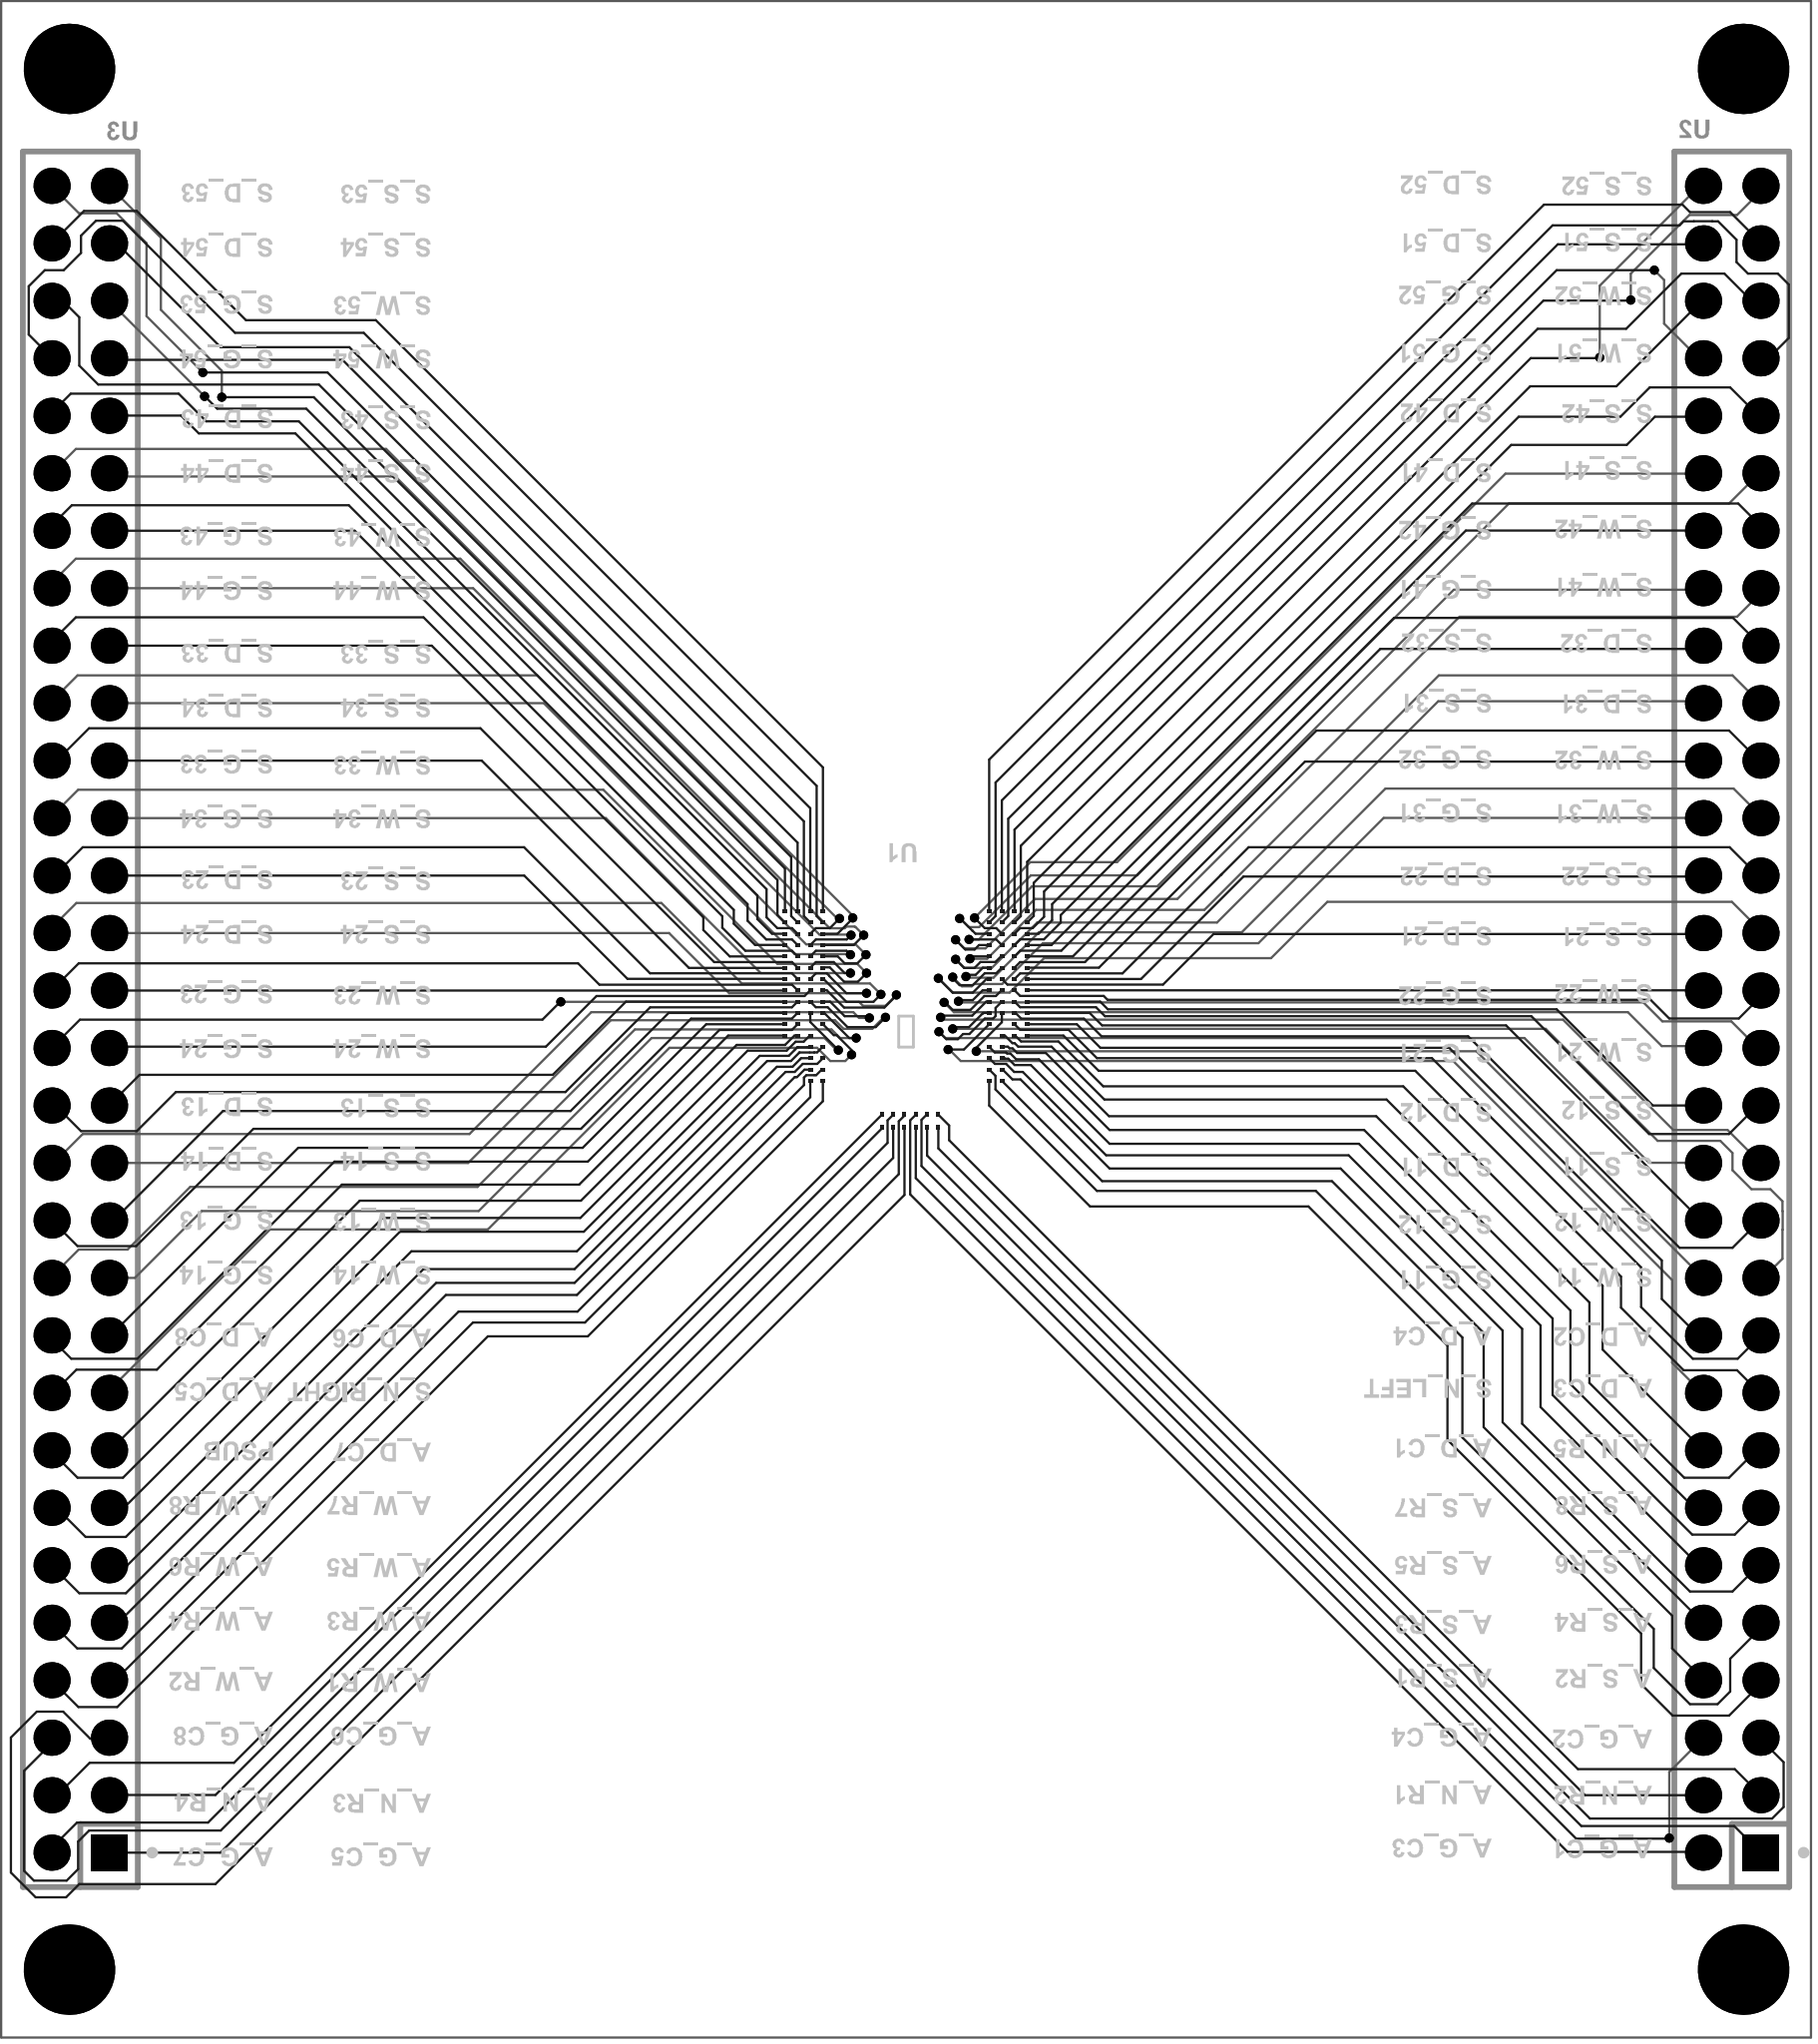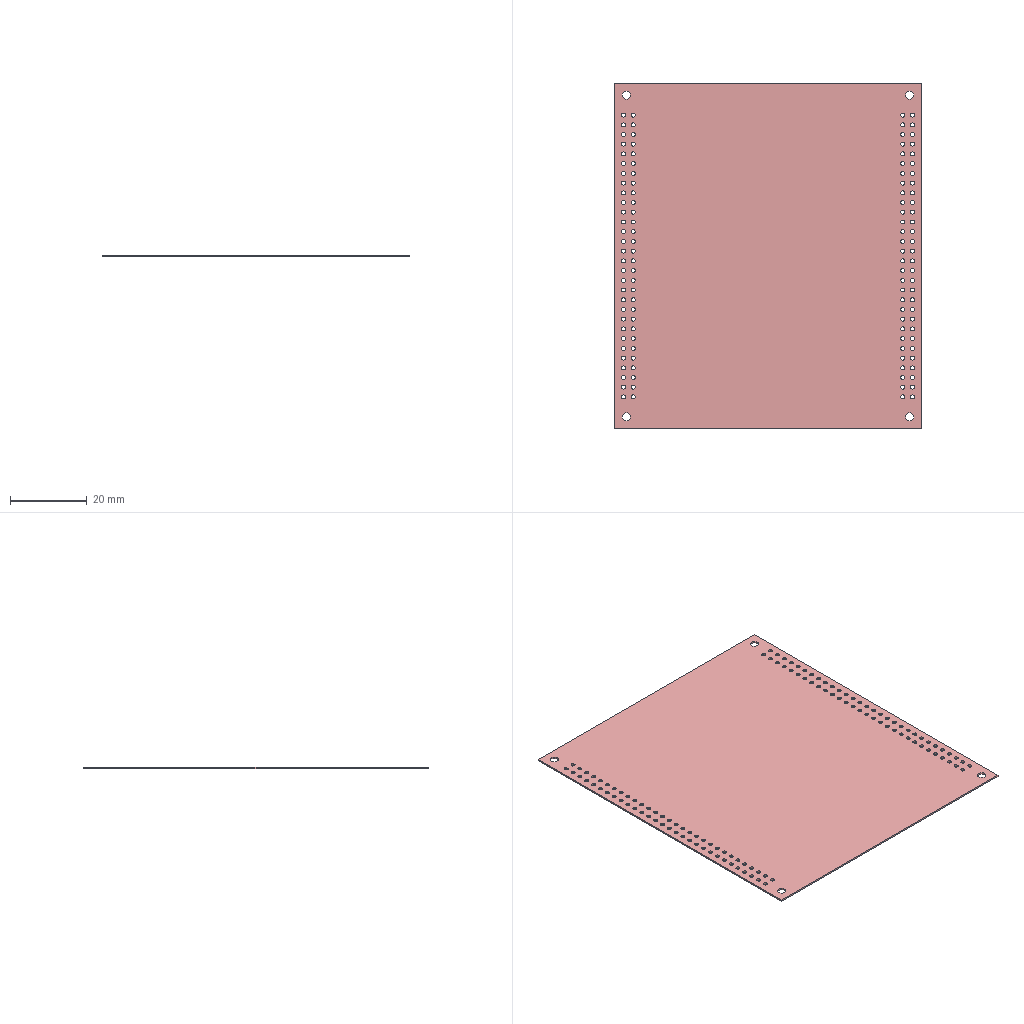Circuit board layout | Altium Designer | box 80 x 90 x 0.4 mm
Layer stack:
# Altium Designer layer stack of  (unit mm; dielectric type: 0 none, 1 core, 2 prepreg, 3 surface material)
index,name,kind,layer,copper_thickness_mm,dielectric_type,dielectric_thickness_mm,dielectric_material,dielectric_constant
0,Top Paste,other,,,,,,
1,Top Overlay,other,,,,,,
2,Top Solder,dielectric,,,3,0.0102,Solder Resist,3.5
3,Top Layer,copper,Top Layer,0.0356,,,,
4,Dielectric1,dielectric,,,0,0.32,FR-4,4.8
5,Bottom Layer,copper,Bottom Layer,0.0356,,,,
6,Bottom Solder,dielectric,,,3,0.0102,Solder Resist,3.5
7,Bottom Overlay,other,,,,,,
8,Bottom Paste,other,,,,,,
# drill layer pairs: low layer,high layer
drill_pair,Top Layer,Bottom Layer
Part placement:
Designator,Comment,Layer,Footprint,Center-X(mm),Center-Y(mm),Rotation
U2,P125-1230A0BS116A1,TopLayer,HDR-TH_60P-P2.54-V-M-R2-C30-S2.54-1,76.5,45,90
U3,P125-1230A0BS116A1,TopLayer,HDR-TH_60P-P2.54-V-M-R2-C30-S2.54-1,3.5,45,90
U1,,TopLayer,XP,40,45,180
Pad and via stacks:
# Altium Designer via and pad stacks of  (unit mm). Each distinct definition once, with the count of objects using it.
# via: kind,start_layer,end_layer,hole_mm,diameter_mm,mode(0 simple;1 top-mid-bottom;2 full stack),diameter_per_layer,count,example_net
# pad: kind,layer,hole_mm,hole_type(0 round;1 square;2 slot),plating,top_size,top_shape(1 round;2 rect;3 octagon;9 rounded rect),mid_size,bottom_size,mode,footprint,size_per_layer,count,example
pad,Multi-Layer,2.2,0,plated,4x4,1,4x4,4x4,0,,,4,0
pad,Multi-Layer,1.05,0,plated,1.6x1.6,1,1.6x1.6,1.6x1.6,0,HDR-TH_60P-P2.54-V-M-R2-C30-S2.54-1,,118,U3.58
pad,Multi-Layer,1.05,0,plated,1.6x1.6,2,1.6x1.6,1.6x1.6,0,HDR-TH_60P-P2.54-V-M-R2-C30-S2.54-1,,2,U3.1
pad,Top Layer,0,0,plated,0.2x0.14,2,0.2x0.14,0.2x0.14,0,XP,,120,U1.101
via,Top Layer,Bottom Layer,0.2032,0.4064,0,,40,S_D_41
Design rules, without the lines most boards share:
# Altium Designer design rules of  (exported by Altium Designer, unit mm)
# columns: name | kind | enabled | priority | scope1 | scope2 | descriptor | typed fields (field=value)
Clearance | 0 | enabled | 1 | All | All | Clearance Constraint (Gap=5mil) (All),(All) | gap=0.127
PlaneConnect | 6 | enabled | 1 | All | All | Power Plane Connect Rule(Relief Connect )(Expansion=20mil) (Conductor Width=10mil) (Air Gap=10mil) (Entries=4) (All) | relief_conductor_width=0.254 relief_entries=4 relief_expansion=0.508
PolygonConnect | 20 | enabled | 1 | All | All | Polygon Connect Rule(Relief Connect )(Conductor Width=10mil) (Relief Angle=90 Angle) (Entries=4) (Air Gap Width=10mil) (All),(All) | connect_style(0=relief,1=direct,2=none)=0 relief_conductor_width=0.254 relief_entries=4
Width | 2 | enabled | 1 | All | All | Width Constraint (Min=4mil) (Max=4mil) (Preferred=4mil) (All) |
RoutingVias | 11 | enabled | 1 | All | All | Routing Via (MinHoleWidth=8mil) (MaxHoleWidth=8mil) (PreferredHoleWidth=8mil) (MinWidth=16mil) (MaxWidth=16mil) (PreferedWidth=16mil) (All) | via_min_hole=0.2032 via_max_hole=0.2032 via_preferred_diameter=0.4064 via_preferred_hole=0.2032
PasteMaskExpansion | 14 | enabled | 1 | All | All | Paste Mask Expansion (Expansion =0mil) (All) | expansion=0
SolderMaskExpansion | 13 | enabled | 1 | All | All | Solder Mask Expansion (Expansion =4mil) (All) | expansion=0.1016
DiffPairsRouting | 51 | enabled | 1 | All | All | Differential Pairs Uncoupled Length using the Gap Constraints (Min=10mil) (Max=10mil) (Prefered=10mil)  and Width Constraints (Min=15mil) (Max=15mil) (Prefered=15mil) (All) |
HoleToHoleClearance | 52 | enabled | 1 | All | All | Hole To Hole Clearance (Gap=10mil) (All),(All) | gap=0.254
MinimumSolderMaskSliver | 53 | enabled | 1 | All | All | Minimum Solder Mask Sliver (Gap=0mil) (All),(All) |
SilkscreenOverComponentPads | 54 | enabled | 1 | IsPad | All | Silk To Solder Mask (Clearance=0mil) (IsPad),(All) |
SilkToSilkClearance | 55 | enabled | 1 | All | All | Silk to Silk (Clearance=0mil) (All),(All) |
Classes set for this board:
# Altium Designer classes of  (member kind: 0 net, 1 component, 2 from-to, 3 pad, 4 layer, 5 differential pair, 6 design channel, 7 polygon, 8 structure, 9 xSignal)
# columns: class name | member kind | superclass | members
1_P1 | 1 | no | U1; U2; U3; U1; U1;